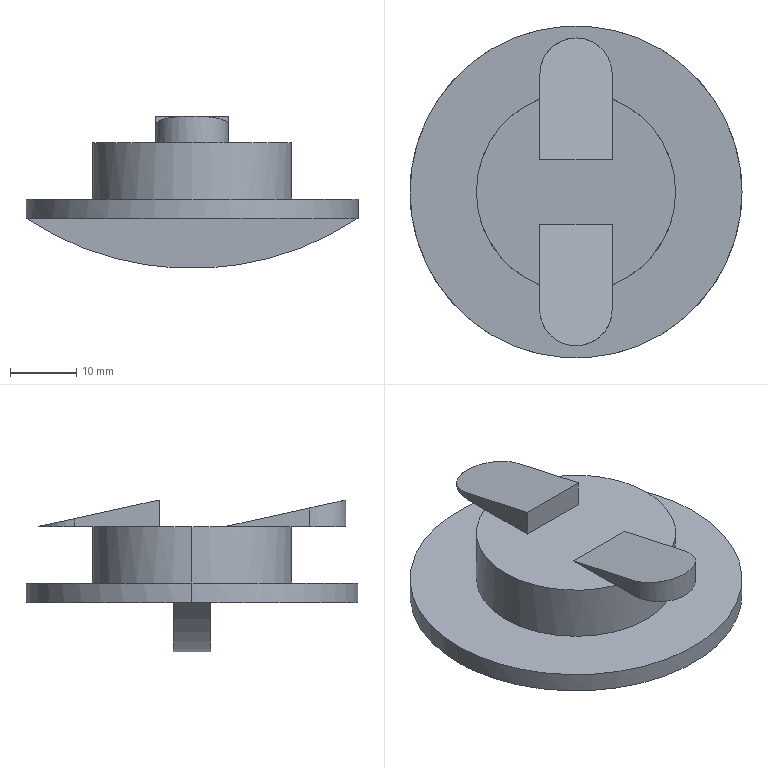Part | SolidWorks | features ICE 5, Extrusion 1 | 1 solid | 25 faces | box 50 x 50 x 22.954 mm | volume 14058 mm3 | plane 17 | cylinder 8 | commonest cylinder face diameters 10.895 x3 30 x2 50 x2 90.233 x1
STEP:
#1=CARTESIAN_POINT('',(15.,0.,10.));
#2=VERTEX_POINT('',#1);
#3=CARTESIAN_POINT('',(5.448,13.976,10.));
#4=VERTEX_POINT('',#3);
#5=CARTESIAN_POINT('',(0.,0.,10.));
#6=DIRECTION('',(0.,0.,1.));
#7=DIRECTION('',(1.,0.,0.));
#8=AXIS2_PLACEMENT_3D('',#5,#6,#7);
#9=CIRCLE('',#8,15.);
#10=EDGE_CURVE('',#2,#4,#9,.T.);
#11=ORIENTED_EDGE('',*,*,#10,.F.);
#12=CARTESIAN_POINT('',(15.,0.,1.5));
#13=VERTEX_POINT('',#12);
#14=CARTESIAN_POINT('',(15.,0.,10.));
#15=DIRECTION('',(0.,0.,-1.));
#16=VECTOR('',#15,1000.);
#17=LINE('',#14,#16);
#18=EDGE_CURVE('',#2,#13,#17,.T.);
#19=ORIENTED_EDGE('',*,*,#18,.T.);
#20=CARTESIAN_POINT('',(-15.,0.,1.5));
#21=VERTEX_POINT('',#20);
#22=CARTESIAN_POINT('',(0.,0.,1.5));
#23=DIRECTION('',(0.,0.,1.));
#24=DIRECTION('',(1.,0.,0.));
#25=AXIS2_PLACEMENT_3D('',#22,#23,#24);
#26=CIRCLE('',#25,15.);
#27=EDGE_CURVE('',#13,#21,#26,.T.);
#28=ORIENTED_EDGE('',*,*,#27,.T.);
#29=CARTESIAN_POINT('',(-15.,0.,10.));
#30=VERTEX_POINT('',#29);
#31=CARTESIAN_POINT('',(-15.,0.,10.));
#32=DIRECTION('',(0.,0.,-1.));
#33=VECTOR('',#32,1000.);
#34=LINE('',#31,#33);
#35=EDGE_CURVE('',#30,#21,#34,.T.);
#36=ORIENTED_EDGE('',*,*,#35,.F.);
#37=CARTESIAN_POINT('',(-5.448,13.976,10.));
#38=VERTEX_POINT('',#37);
#39=CARTESIAN_POINT('',(0.,0.,10.));
#40=DIRECTION('',(0.,0.,1.));
#41=DIRECTION('',(1.,0.,0.));
#42=AXIS2_PLACEMENT_3D('',#39,#40,#41);
#43=CIRCLE('',#42,15.);
#44=EDGE_CURVE('',#38,#30,#43,.T.);
#45=ORIENTED_EDGE('',*,*,#44,.F.);
#46=CARTESIAN_POINT('',(0.,0.,10.));
#47=DIRECTION('',(0.,0.,1.));
#48=DIRECTION('',(1.,0.,0.));
#49=AXIS2_PLACEMENT_3D('',#46,#47,#48);
#50=CIRCLE('',#49,15.);
#51=EDGE_CURVE('',#4,#38,#50,.T.);
#52=ORIENTED_EDGE('',*,*,#51,.F.);
#53=EDGE_LOOP('',(#11,#19,#28,#36,#45,#52));
#54=FACE_OUTER_BOUND('',#53,.T.);
#55=CARTESIAN_POINT('',(0.,0.,10.));
#56=DIRECTION('',(0.,0.,-1.));
#57=DIRECTION('',(-1.,0.,0.));
#58=AXIS2_PLACEMENT_3D('',#55,#56,#57);
#59=CYLINDRICAL_SURFACE('',#58,15.);
#60=ADVANCED_FACE('',(#54),#59,.T.);
#61=CARTESIAN_POINT('',(25.,0.,1.5));
#62=VERTEX_POINT('',#61);
#63=CARTESIAN_POINT('',(-25.,0.,1.5));
#64=VERTEX_POINT('',#63);
#65=CARTESIAN_POINT('',(0.,0.,1.5));
#66=DIRECTION('',(0.,0.,1.));
#67=DIRECTION('',(1.,0.,0.));
#68=AXIS2_PLACEMENT_3D('',#65,#66,#67);
#69=CIRCLE('',#68,25.);
#70=EDGE_CURVE('',#62,#64,#69,.T.);
#71=ORIENTED_EDGE('',*,*,#70,.F.);
#72=CARTESIAN_POINT('',(25.,0.,-1.5));
#73=VERTEX_POINT('',#72);
#74=CARTESIAN_POINT('',(25.,0.,1.5));
#75=DIRECTION('',(0.,0.,-1.));
#76=VECTOR('',#75,1000.);
#77=LINE('',#74,#76);
#78=EDGE_CURVE('',#62,#73,#77,.T.);
#79=ORIENTED_EDGE('',*,*,#78,.T.);
#80=CARTESIAN_POINT('',(24.841,2.817,-1.5));
#81=VERTEX_POINT('',#80);
#82=CARTESIAN_POINT('',(0.,0.,-1.5));
#83=DIRECTION('',(0.,0.,1.));
#84=DIRECTION('',(1.,0.,0.));
#85=AXIS2_PLACEMENT_3D('',#82,#83,#84);
#86=CIRCLE('',#85,25.);
#87=EDGE_CURVE('',#73,#81,#86,.T.);
#88=ORIENTED_EDGE('',*,*,#87,.T.);
#89=CARTESIAN_POINT('',(-24.841,2.817,-1.5));
#90=VERTEX_POINT('',#89);
#91=CARTESIAN_POINT('',(0.,0.,-1.5));
#92=DIRECTION('',(0.,0.,1.));
#93=DIRECTION('',(1.,0.,0.));
#94=AXIS2_PLACEMENT_3D('',#91,#92,#93);
#95=CIRCLE('',#94,25.);
#96=EDGE_CURVE('',#81,#90,#95,.T.);
#97=ORIENTED_EDGE('',*,*,#96,.T.);
#98=CARTESIAN_POINT('',(-25.,0.,-1.5));
#99=VERTEX_POINT('',#98);
#100=CARTESIAN_POINT('',(0.,0.,-1.5));
#101=DIRECTION('',(0.,0.,1.));
#102=DIRECTION('',(1.,0.,0.));
#103=AXIS2_PLACEMENT_3D('',#100,#101,#102);
#104=CIRCLE('',#103,25.);
#105=EDGE_CURVE('',#90,#99,#104,.T.);
#106=ORIENTED_EDGE('',*,*,#105,.T.);
#107=CARTESIAN_POINT('',(-25.,0.,1.5));
#108=DIRECTION('',(0.,0.,-1.));
#109=VECTOR('',#108,1000.);
#110=LINE('',#107,#109);
#111=EDGE_CURVE('',#64,#99,#110,.T.);
#112=ORIENTED_EDGE('',*,*,#111,.F.);
#113=EDGE_LOOP('',(#71,#79,#88,#97,#106,#112));
#114=FACE_OUTER_BOUND('',#113,.T.);
#115=CARTESIAN_POINT('',(0.,0.,1.5));
#116=DIRECTION('',(0.,0.,-1.));
#117=DIRECTION('',(-1.,0.,0.));
#118=AXIS2_PLACEMENT_3D('',#115,#116,#117);
#119=CYLINDRICAL_SURFACE('',#118,25.);
#120=ADVANCED_FACE('',(#114),#119,.T.);
#121=CARTESIAN_POINT('',(5.448,17.731,10.));
#122=VERTEX_POINT('',#121);
#123=CARTESIAN_POINT('',(0.,23.178,10.));
#124=VERTEX_POINT('',#123);
#125=CARTESIAN_POINT('',(0.,17.731,10.));
#126=DIRECTION('',(0.,0.,1.));
#127=DIRECTION('',(-1.,0.,0.));
#128=AXIS2_PLACEMENT_3D('',#125,#126,#127);
#129=CIRCLE('',#128,5.448);
#130=EDGE_CURVE('',#122,#124,#129,.T.);
#131=ORIENTED_EDGE('',*,*,#130,.T.);
#132=CARTESIAN_POINT('',(5.448,17.731,11.195));
#133=VERTEX_POINT('',#132);
#134=CARTESIAN_POINT('',(0.,23.178,10.));
#135=CARTESIAN_POINT('',(3.191,23.178,10.));
#136=CARTESIAN_POINT('',(5.448,20.922,10.495));
#137=CARTESIAN_POINT('',(5.448,17.731,11.195));
#138=(BOUNDED_CURVE()B_SPLINE_CURVE(3,(#134,#135,#136,#137),.UNSPECIFIED.,.F.,.F.)B_SPLINE_CURVE_WITH_KNOTS((4,4),(0.,1.571),.UNSPECIFIED.)CURVE()GEOMETRIC_REPRESENTATION_ITEM()RATIONAL_B_SPLINE_CURVE((1.,0.8047,0.8047,1.))REPRESENTATION_ITEM(''));
#139=EDGE_CURVE('',#124,#133,#138,.T.);
#140=ORIENTED_EDGE('',*,*,#139,.T.);
#141=CARTESIAN_POINT('',(5.448,17.731,14.));
#142=DIRECTION('',(0.,0.,-1.));
#143=VECTOR('',#142,1000.);
#144=LINE('',#141,#143);
#145=EDGE_CURVE('',#133,#122,#144,.T.);
#146=ORIENTED_EDGE('',*,*,#145,.T.);
#147=EDGE_LOOP('',(#131,#140,#146));
#148=FACE_OUTER_BOUND('',#147,.T.);
#149=CARTESIAN_POINT('',(0.,17.731,14.));
#150=DIRECTION('',(0.,0.,-1.));
#151=DIRECTION('',(-1.,0.,0.));
#152=AXIS2_PLACEMENT_3D('',#149,#150,#151);
#153=CYLINDRICAL_SURFACE('',#152,5.448);
#154=ADVANCED_FACE('',(#148),#153,.T.);
#155=CARTESIAN_POINT('',(5.448,-4.944,10.));
#156=VERTEX_POINT('',#155);
#157=CARTESIAN_POINT('',(-5.448,-4.944,10.));
#158=VERTEX_POINT('',#157);
#159=CARTESIAN_POINT('',(-5.448,-4.944,10.));
#160=DIRECTION('',(-1.,0.,0.));
#161=VECTOR('',#160,1000.);
#162=LINE('',#159,#161);
#163=EDGE_CURVE('',#156,#158,#162,.T.);
#164=ORIENTED_EDGE('',*,*,#163,.F.);
#165=CARTESIAN_POINT('',(5.448,-13.976,10.));
#166=VERTEX_POINT('',#165);
#167=CARTESIAN_POINT('',(5.448,0.,10.));
#168=DIRECTION('',(0.,-1.,0.));
#169=VECTOR('',#168,1000.);
#170=LINE('',#167,#169);
#171=EDGE_CURVE('',#156,#166,#170,.T.);
#172=ORIENTED_EDGE('',*,*,#171,.T.);
#173=CARTESIAN_POINT('',(0.,0.,10.));
#174=DIRECTION('',(0.,0.,1.));
#175=DIRECTION('',(1.,0.,0.));
#176=AXIS2_PLACEMENT_3D('',#173,#174,#175);
#177=CIRCLE('',#176,15.);
#178=EDGE_CURVE('',#166,#2,#177,.T.);
#179=ORIENTED_EDGE('',*,*,#178,.T.);
#180=ORIENTED_EDGE('',*,*,#10,.T.);
#181=CARTESIAN_POINT('',(5.448,4.944,10.));
#182=VERTEX_POINT('',#181);
#183=CARTESIAN_POINT('',(5.448,17.731,10.));
#184=DIRECTION('',(0.,1.,0.));
#185=VECTOR('',#184,1000.);
#186=LINE('',#183,#185);
#187=EDGE_CURVE('',#182,#4,#186,.T.);
#188=ORIENTED_EDGE('',*,*,#187,.F.);
#189=CARTESIAN_POINT('',(-5.448,4.944,10.));
#190=VERTEX_POINT('',#189);
#191=CARTESIAN_POINT('',(-5.448,4.944,10.));
#192=DIRECTION('',(1.,0.,0.));
#193=VECTOR('',#192,1000.);
#194=LINE('',#191,#193);
#195=EDGE_CURVE('',#190,#182,#194,.T.);
#196=ORIENTED_EDGE('',*,*,#195,.F.);
#197=CARTESIAN_POINT('',(-5.448,17.731,10.));
#198=DIRECTION('',(0.,-1.,0.));
#199=VECTOR('',#198,1000.);
#200=LINE('',#197,#199);
#201=EDGE_CURVE('',#38,#190,#200,.T.);
#202=ORIENTED_EDGE('',*,*,#201,.F.);
#203=ORIENTED_EDGE('',*,*,#44,.T.);
#204=CARTESIAN_POINT('',(-5.448,-13.976,10.));
#205=VERTEX_POINT('',#204);
#206=CARTESIAN_POINT('',(0.,0.,10.));
#207=DIRECTION('',(0.,0.,1.));
#208=DIRECTION('',(1.,0.,0.));
#209=AXIS2_PLACEMENT_3D('',#206,#207,#208);
#210=CIRCLE('',#209,15.);
#211=EDGE_CURVE('',#30,#205,#210,.T.);
#212=ORIENTED_EDGE('',*,*,#211,.T.);
#213=CARTESIAN_POINT('',(-5.448,-17.731,10.));
#214=DIRECTION('',(0.,-1.,0.));
#215=VECTOR('',#214,1000.);
#216=LINE('',#213,#215);
#217=EDGE_CURVE('',#158,#205,#216,.T.);
#218=ORIENTED_EDGE('',*,*,#217,.F.);
#219=EDGE_LOOP('',(#164,#172,#179,#180,#188,#196,#202,#203,#212,#218));
#220=FACE_OUTER_BOUND('',#219,.T.);
#221=CARTESIAN_POINT('',(0.,0.,10.));
#222=DIRECTION('',(0.,0.,1.));
#223=DIRECTION('',(1.,0.,0.));
#224=AXIS2_PLACEMENT_3D('',#221,#222,#223);
#225=PLANE('',#224);
#226=ADVANCED_FACE('',(#220),#225,.T.);
#227=CARTESIAN_POINT('',(24.841,-2.817,-1.5));
#228=VERTEX_POINT('',#227);
#229=CARTESIAN_POINT('',(-24.841,-2.817,-1.5));
#230=VERTEX_POINT('',#229);
#231=CARTESIAN_POINT('',(0.,-2.817,-1.5));
#232=DIRECTION('',(-1.,0.,0.));
#233=VECTOR('',#232,1000.);
#234=LINE('',#231,#233);
#235=EDGE_CURVE('',#228,#230,#234,.T.);
#236=ORIENTED_EDGE('',*,*,#235,.T.);
#237=CARTESIAN_POINT('',(0.,-2.817,36.162));
#238=DIRECTION('',(0.,-1.,0.));
#239=DIRECTION('',(-1.,0.,0.));
#240=AXIS2_PLACEMENT_3D('',#237,#238,#239);
#241=CIRCLE('',#240,45.116);
#242=EDGE_CURVE('',#230,#228,#241,.T.);
#243=ORIENTED_EDGE('',*,*,#242,.T.);
#244=EDGE_LOOP('',(#236,#243));
#245=FACE_OUTER_BOUND('',#244,.T.);
#246=CARTESIAN_POINT('',(0.,-2.817,-9.5));
#247=DIRECTION('',(0.,1.,0.));
#248=DIRECTION('',(-1.,0.,0.));
#249=AXIS2_PLACEMENT_3D('',#246,#247,#248);
#250=PLANE('',#249);
#251=ADVANCED_FACE('',(#245),#250,.F.);
#252=CARTESIAN_POINT('',(0.,2.817,36.162));
#253=DIRECTION('',(0.,-1.,0.));
#254=DIRECTION('',(-1.,0.,0.));
#255=AXIS2_PLACEMENT_3D('',#252,#253,#254);
#256=CIRCLE('',#255,45.116);
#257=EDGE_CURVE('',#90,#81,#256,.T.);
#258=ORIENTED_EDGE('',*,*,#257,.F.);
#259=CARTESIAN_POINT('',(0.,2.817,-1.5));
#260=DIRECTION('',(-1.,0.,0.));
#261=VECTOR('',#260,1000.);
#262=LINE('',#259,#261);
#263=EDGE_CURVE('',#81,#90,#262,.T.);
#264=ORIENTED_EDGE('',*,*,#263,.F.);
#265=EDGE_LOOP('',(#258,#264));
#266=FACE_OUTER_BOUND('',#265,.T.);
#267=CARTESIAN_POINT('',(0.,2.817,-9.5));
#268=DIRECTION('',(0.,1.,0.));
#269=DIRECTION('',(-1.,0.,0.));
#270=AXIS2_PLACEMENT_3D('',#267,#268,#269);
#271=PLANE('',#270);
#272=ADVANCED_FACE('',(#266),#271,.T.);
#273=ORIENTED_EDGE('',*,*,#235,.F.);
#274=CARTESIAN_POINT('',(0.,0.,-1.5));
#275=DIRECTION('',(0.,0.,1.));
#276=DIRECTION('',(1.,0.,0.));
#277=AXIS2_PLACEMENT_3D('',#274,#275,#276);
#278=CIRCLE('',#277,25.);
#279=EDGE_CURVE('',#230,#228,#278,.T.);
#280=ORIENTED_EDGE('',*,*,#279,.F.);
#281=EDGE_LOOP('',(#273,#280));
#282=FACE_OUTER_BOUND('',#281,.T.);
#283=CARTESIAN_POINT('',(0.,0.,-1.5));
#284=DIRECTION('',(0.,0.,1.));
#285=DIRECTION('',(1.,0.,0.));
#286=AXIS2_PLACEMENT_3D('',#283,#284,#285);
#287=PLANE('',#286);
#288=ADVANCED_FACE('',(#282),#287,.F.);
#289=ORIENTED_EDGE('',*,*,#78,.F.);
#290=CARTESIAN_POINT('',(0.,0.,1.5));
#291=DIRECTION('',(0.,0.,1.));
#292=DIRECTION('',(1.,0.,0.));
#293=AXIS2_PLACEMENT_3D('',#290,#291,#292);
#294=CIRCLE('',#293,25.);
#295=EDGE_CURVE('',#64,#62,#294,.T.);
#296=ORIENTED_EDGE('',*,*,#295,.F.);
#297=ORIENTED_EDGE('',*,*,#111,.T.);
#298=CARTESIAN_POINT('',(0.,0.,-1.5));
#299=DIRECTION('',(0.,0.,1.));
#300=DIRECTION('',(1.,0.,0.));
#301=AXIS2_PLACEMENT_3D('',#298,#299,#300);
#302=CIRCLE('',#301,25.);
#303=EDGE_CURVE('',#99,#230,#302,.T.);
#304=ORIENTED_EDGE('',*,*,#303,.T.);
#305=ORIENTED_EDGE('',*,*,#279,.T.);
#306=CARTESIAN_POINT('',(0.,0.,-1.5));
#307=DIRECTION('',(0.,0.,1.));
#308=DIRECTION('',(1.,0.,0.));
#309=AXIS2_PLACEMENT_3D('',#306,#307,#308);
#310=CIRCLE('',#309,25.);
#311=EDGE_CURVE('',#228,#73,#310,.T.);
#312=ORIENTED_EDGE('',*,*,#311,.T.);
#313=EDGE_LOOP('',(#289,#296,#297,#304,#305,#312));
#314=FACE_OUTER_BOUND('',#313,.T.);
#315=CARTESIAN_POINT('',(0.,0.,1.5));
#316=DIRECTION('',(0.,0.,-1.));
#317=DIRECTION('',(-1.,0.,0.));
#318=AXIS2_PLACEMENT_3D('',#315,#316,#317);
#319=CYLINDRICAL_SURFACE('',#318,25.);
#320=ADVANCED_FACE('',(#314),#319,.T.);
#321=CARTESIAN_POINT('',(0.,0.,1.5));
#322=DIRECTION('',(0.,0.,1.));
#323=DIRECTION('',(1.,0.,0.));
#324=AXIS2_PLACEMENT_3D('',#321,#322,#323);
#325=CIRCLE('',#324,15.);
#326=EDGE_CURVE('',#21,#13,#325,.T.);
#327=ORIENTED_EDGE('',*,*,#326,.F.);
#328=ORIENTED_EDGE('',*,*,#27,.F.);
#329=EDGE_LOOP('',(#327,#328));
#330=FACE_BOUND('',#329,.T.);
#331=ORIENTED_EDGE('',*,*,#295,.T.);
#332=ORIENTED_EDGE('',*,*,#70,.T.);
#333=EDGE_LOOP('',(#331,#332));
#334=FACE_OUTER_BOUND('',#333,.T.);
#335=CARTESIAN_POINT('',(0.,0.,1.5));
#336=DIRECTION('',(0.,0.,1.));
#337=DIRECTION('',(1.,0.,0.));
#338=AXIS2_PLACEMENT_3D('',#335,#336,#337);
#339=PLANE('',#338);
#340=ADVANCED_FACE('',(#330,#334),#339,.T.);
#341=ORIENTED_EDGE('',*,*,#96,.F.);
#342=ORIENTED_EDGE('',*,*,#263,.T.);
#343=EDGE_LOOP('',(#341,#342));
#344=FACE_OUTER_BOUND('',#343,.T.);
#345=CARTESIAN_POINT('',(0.,0.,-1.5));
#346=DIRECTION('',(0.,0.,1.));
#347=DIRECTION('',(1.,0.,0.));
#348=AXIS2_PLACEMENT_3D('',#345,#346,#347);
#349=PLANE('',#348);
#350=ADVANCED_FACE('',(#344),#349,.F.);
#351=CARTESIAN_POINT('',(-24.841,-5.183,-1.5));
#352=DIRECTION('',(0.,1.,0.));
#353=VECTOR('',#352,1000.);
#354=LINE('',#351,#353);
#355=EDGE_CURVE('',#230,#90,#354,.T.);
#356=ORIENTED_EDGE('',*,*,#355,.F.);
#357=ORIENTED_EDGE('',*,*,#303,.F.);
#358=ORIENTED_EDGE('',*,*,#105,.F.);
#359=EDGE_LOOP('',(#356,#357,#358));
#360=FACE_OUTER_BOUND('',#359,.T.);
#361=CARTESIAN_POINT('',(0.,-5.183,-1.5));
#362=DIRECTION('',(0.,0.,1.));
#363=DIRECTION('',(1.,0.,0.));
#364=AXIS2_PLACEMENT_3D('',#361,#362,#363);
#365=PLANE('',#364);
#366=ADVANCED_FACE('',(#360),#365,.F.);
#367=CARTESIAN_POINT('',(24.841,-5.183,-1.5));
#368=DIRECTION('',(0.,1.,0.));
#369=VECTOR('',#368,1000.);
#370=LINE('',#367,#369);
#371=EDGE_CURVE('',#228,#81,#370,.T.);
#372=ORIENTED_EDGE('',*,*,#371,.T.);
#373=ORIENTED_EDGE('',*,*,#87,.F.);
#374=ORIENTED_EDGE('',*,*,#311,.F.);
#375=EDGE_LOOP('',(#372,#373,#374));
#376=FACE_OUTER_BOUND('',#375,.T.);
#377=CARTESIAN_POINT('',(0.,-5.183,-1.5));
#378=DIRECTION('',(0.,0.,1.));
#379=DIRECTION('',(1.,0.,0.));
#380=AXIS2_PLACEMENT_3D('',#377,#378,#379);
#381=PLANE('',#380);
#382=ADVANCED_FACE('',(#376),#381,.F.);
#383=ORIENTED_EDGE('',*,*,#355,.T.);
#384=ORIENTED_EDGE('',*,*,#257,.T.);
#385=ORIENTED_EDGE('',*,*,#371,.F.);
#386=ORIENTED_EDGE('',*,*,#242,.F.);
#387=EDGE_LOOP('',(#383,#384,#385,#386));
#388=FACE_OUTER_BOUND('',#387,.T.);
#389=CARTESIAN_POINT('',(0.,-5.183,36.162));
#390=DIRECTION('',(0.,1.,0.));
#391=DIRECTION('',(-1.,0.,0.));
#392=AXIS2_PLACEMENT_3D('',#389,#390,#391);
#393=CYLINDRICAL_SURFACE('',#392,45.116);
#394=ADVANCED_FACE('',(#388),#393,.T.);
#395=ORIENTED_EDGE('',*,*,#18,.F.);
#396=ORIENTED_EDGE('',*,*,#178,.F.);
#397=CARTESIAN_POINT('',(0.,0.,10.));
#398=DIRECTION('',(0.,0.,1.));
#399=DIRECTION('',(1.,0.,0.));
#400=AXIS2_PLACEMENT_3D('',#397,#398,#399);
#401=CIRCLE('',#400,15.);
#402=EDGE_CURVE('',#205,#166,#401,.T.);
#403=ORIENTED_EDGE('',*,*,#402,.F.);
#404=ORIENTED_EDGE('',*,*,#211,.F.);
#405=ORIENTED_EDGE('',*,*,#35,.T.);
#406=ORIENTED_EDGE('',*,*,#326,.T.);
#407=EDGE_LOOP('',(#395,#396,#403,#404,#405,#406));
#408=FACE_OUTER_BOUND('',#407,.T.);
#409=CARTESIAN_POINT('',(0.,0.,10.));
#410=DIRECTION('',(0.,0.,-1.));
#411=DIRECTION('',(-1.,0.,0.));
#412=AXIS2_PLACEMENT_3D('',#409,#410,#411);
#413=CYLINDRICAL_SURFACE('',#412,15.);
#414=ADVANCED_FACE('',(#408),#413,.T.);
#415=ORIENTED_EDGE('',*,*,#145,.F.);
#416=CARTESIAN_POINT('',(5.448,4.944,14.));
#417=VERTEX_POINT('',#416);
#418=CARTESIAN_POINT('',(5.448,17.144,11.324));
#419=DIRECTION('',(0.,-0.9768,0.2143));
#420=VECTOR('',#419,1000.);
#421=LINE('',#418,#420);
#422=EDGE_CURVE('',#133,#417,#421,.T.);
#423=ORIENTED_EDGE('',*,*,#422,.T.);
#424=CARTESIAN_POINT('',(5.448,4.944,14.));
#425=DIRECTION('',(0.,0.,-1.));
#426=VECTOR('',#425,1000.);
#427=LINE('',#424,#426);
#428=EDGE_CURVE('',#417,#182,#427,.T.);
#429=ORIENTED_EDGE('',*,*,#428,.T.);
#430=ORIENTED_EDGE('',*,*,#187,.T.);
#431=CARTESIAN_POINT('',(5.448,17.731,10.));
#432=DIRECTION('',(0.,1.,0.));
#433=VECTOR('',#432,1000.);
#434=LINE('',#431,#433);
#435=EDGE_CURVE('',#4,#122,#434,.T.);
#436=ORIENTED_EDGE('',*,*,#435,.T.);
#437=EDGE_LOOP('',(#415,#423,#429,#430,#436));
#438=FACE_OUTER_BOUND('',#437,.T.);
#439=CARTESIAN_POINT('',(5.448,17.731,14.));
#440=DIRECTION('',(-1.,0.,0.));
#441=DIRECTION('',(0.,-1.,0.));
#442=AXIS2_PLACEMENT_3D('',#439,#440,#441);
#443=PLANE('',#442);
#444=ADVANCED_FACE('',(#438),#443,.F.);
#445=CARTESIAN_POINT('',(-5.448,17.731,11.195));
#446=VERTEX_POINT('',#445);
#447=CARTESIAN_POINT('',(-5.448,17.731,10.));
#448=VERTEX_POINT('',#447);
#449=CARTESIAN_POINT('',(-5.448,17.731,14.));
#450=DIRECTION('',(0.,0.,-1.));
#451=VECTOR('',#450,1000.);
#452=LINE('',#449,#451);
#453=EDGE_CURVE('',#446,#448,#452,.T.);
#454=ORIENTED_EDGE('',*,*,#453,.F.);
#455=CARTESIAN_POINT('',(-5.448,17.731,11.195));
#456=CARTESIAN_POINT('',(-5.448,20.922,10.495));
#457=CARTESIAN_POINT('',(-3.191,23.178,10.));
#458=CARTESIAN_POINT('',(0.,23.178,10.));
#459=(BOUNDED_CURVE()B_SPLINE_CURVE(3,(#455,#456,#457,#458),.UNSPECIFIED.,.F.,.F.)B_SPLINE_CURVE_WITH_KNOTS((4,4),(4.712,6.283),.UNSPECIFIED.)CURVE()GEOMETRIC_REPRESENTATION_ITEM()RATIONAL_B_SPLINE_CURVE((1.,0.8047,0.8047,1.))REPRESENTATION_ITEM(''));
#460=EDGE_CURVE('',#446,#124,#459,.T.);
#461=ORIENTED_EDGE('',*,*,#460,.T.);
#462=CARTESIAN_POINT('',(0.,17.731,10.));
#463=DIRECTION('',(0.,0.,1.));
#464=DIRECTION('',(-1.,0.,0.));
#465=AXIS2_PLACEMENT_3D('',#462,#463,#464);
#466=CIRCLE('',#465,5.448);
#467=EDGE_CURVE('',#124,#448,#466,.T.);
#468=ORIENTED_EDGE('',*,*,#467,.T.);
#469=EDGE_LOOP('',(#454,#461,#468));
#470=FACE_OUTER_BOUND('',#469,.T.);
#471=CARTESIAN_POINT('',(0.,17.731,14.));
#472=DIRECTION('',(0.,0.,-1.));
#473=DIRECTION('',(-1.,0.,0.));
#474=AXIS2_PLACEMENT_3D('',#471,#472,#473);
#475=CYLINDRICAL_SURFACE('',#474,5.448);
#476=ADVANCED_FACE('',(#470),#475,.T.);
#477=CARTESIAN_POINT('',(-5.448,4.944,14.));
#478=VERTEX_POINT('',#477);
#479=CARTESIAN_POINT('',(-5.448,4.944,14.));
#480=DIRECTION('',(0.,0.,-1.));
#481=VECTOR('',#480,1000.);
#482=LINE('',#479,#481);
#483=EDGE_CURVE('',#478,#190,#482,.T.);
#484=ORIENTED_EDGE('',*,*,#483,.F.);
#485=CARTESIAN_POINT('',(-5.448,23.178,10.));
#486=DIRECTION('',(0.,-0.9768,0.2143));
#487=VECTOR('',#486,1000.);
#488=LINE('',#485,#487);
#489=EDGE_CURVE('',#446,#478,#488,.T.);
#490=ORIENTED_EDGE('',*,*,#489,.F.);
#491=ORIENTED_EDGE('',*,*,#453,.T.);
#492=CARTESIAN_POINT('',(-5.448,17.731,10.));
#493=DIRECTION('',(0.,-1.,0.));
#494=VECTOR('',#493,1000.);
#495=LINE('',#492,#494);
#496=EDGE_CURVE('',#448,#38,#495,.T.);
#497=ORIENTED_EDGE('',*,*,#496,.T.);
#498=ORIENTED_EDGE('',*,*,#201,.T.);
#499=EDGE_LOOP('',(#484,#490,#491,#497,#498));
#500=FACE_OUTER_BOUND('',#499,.T.);
#501=CARTESIAN_POINT('',(-5.448,17.731,14.));
#502=DIRECTION('',(1.,0.,0.));
#503=DIRECTION('',(0.,1.,0.));
#504=AXIS2_PLACEMENT_3D('',#501,#502,#503);
#505=PLANE('',#504);
#506=ADVANCED_FACE('',(#500),#505,.F.);
#507=ORIENTED_EDGE('',*,*,#195,.T.);
#508=ORIENTED_EDGE('',*,*,#428,.F.);
#509=CARTESIAN_POINT('',(-5.448,4.944,14.));
#510=DIRECTION('',(1.,0.,0.));
#511=VECTOR('',#510,1000.);
#512=LINE('',#509,#511);
#513=EDGE_CURVE('',#478,#417,#512,.T.);
#514=ORIENTED_EDGE('',*,*,#513,.F.);
#515=ORIENTED_EDGE('',*,*,#483,.T.);
#516=EDGE_LOOP('',(#507,#508,#514,#515));
#517=FACE_OUTER_BOUND('',#516,.T.);
#518=CARTESIAN_POINT('',(-5.448,4.944,14.));
#519=DIRECTION('',(0.,1.,0.));
#520=DIRECTION('',(0.,0.,1.));
#521=AXIS2_PLACEMENT_3D('',#518,#519,#520);
#522=PLANE('',#521);
#523=ADVANCED_FACE('',(#517),#522,.F.);
#524=ORIENTED_EDGE('',*,*,#435,.F.);
#525=ORIENTED_EDGE('',*,*,#51,.T.);
#526=ORIENTED_EDGE('',*,*,#496,.F.);
#527=ORIENTED_EDGE('',*,*,#467,.F.);
#528=ORIENTED_EDGE('',*,*,#130,.F.);
#529=EDGE_LOOP('',(#524,#525,#526,#527,#528));
#530=FACE_OUTER_BOUND('',#529,.T.);
#531=CARTESIAN_POINT('',(0.,17.731,10.));
#532=DIRECTION('',(0.,0.,-1.));
#533=DIRECTION('',(-1.,0.,0.));
#534=AXIS2_PLACEMENT_3D('',#531,#532,#533);
#535=PLANE('',#534);
#536=ADVANCED_FACE('',(#530),#535,.T.);
#537=CARTESIAN_POINT('',(5.448,-17.731,12.805));
#538=VERTEX_POINT('',#537);
#539=CARTESIAN_POINT('',(5.448,-17.731,10.));
#540=VERTEX_POINT('',#539);
#541=CARTESIAN_POINT('',(5.448,-17.731,14.));
#542=DIRECTION('',(0.,0.,-1.));
#543=VECTOR('',#542,1000.);
#544=LINE('',#541,#543);
#545=EDGE_CURVE('',#538,#540,#544,.T.);
#546=ORIENTED_EDGE('',*,*,#545,.F.);
#547=CARTESIAN_POINT('',(-5.448,-17.731,12.805));
#548=VERTEX_POINT('',#547);
#549=CARTESIAN_POINT('',(5.448,-17.731,12.805));
#550=CARTESIAN_POINT('',(5.448,-28.626,15.195));
#551=CARTESIAN_POINT('',(-5.448,-28.626,15.195));
#552=CARTESIAN_POINT('',(-5.448,-17.731,12.805));
#553=(BOUNDED_CURVE()B_SPLINE_CURVE(3,(#549,#550,#551,#552),.UNSPECIFIED.,.F.,.F.)B_SPLINE_CURVE_WITH_KNOTS((4,4),(1.571,4.712),.UNSPECIFIED.)CURVE()GEOMETRIC_REPRESENTATION_ITEM()RATIONAL_B_SPLINE_CURVE((1.,0.3333,0.3333,1.))REPRESENTATION_ITEM(''));
#554=EDGE_CURVE('',#538,#548,#553,.T.);
#555=ORIENTED_EDGE('',*,*,#554,.T.);
#556=CARTESIAN_POINT('',(-5.448,-17.731,10.));
#557=VERTEX_POINT('',#556);
#558=CARTESIAN_POINT('',(-5.448,-17.731,14.));
#559=DIRECTION('',(0.,0.,-1.));
#560=VECTOR('',#559,1000.);
#561=LINE('',#558,#560);
#562=EDGE_CURVE('',#548,#557,#561,.T.);
#563=ORIENTED_EDGE('',*,*,#562,.T.);
#564=CARTESIAN_POINT('',(0.,-17.731,10.));
#565=DIRECTION('',(0.,0.,1.));
#566=DIRECTION('',(1.,0.,0.));
#567=AXIS2_PLACEMENT_3D('',#564,#565,#566);
#568=CIRCLE('',#567,5.448);
#569=EDGE_CURVE('',#557,#540,#568,.T.);
#570=ORIENTED_EDGE('',*,*,#569,.T.);
#571=EDGE_LOOP('',(#546,#555,#563,#570));
#572=FACE_OUTER_BOUND('',#571,.T.);
#573=CARTESIAN_POINT('',(0.,-17.731,14.));
#574=DIRECTION('',(0.,0.,-1.));
#575=DIRECTION('',(-1.,0.,0.));
#576=AXIS2_PLACEMENT_3D('',#573,#574,#575);
#577=CYLINDRICAL_SURFACE('',#576,5.448);
#578=ADVANCED_FACE('',(#572),#577,.T.);
#579=ORIENTED_EDGE('',*,*,#171,.F.);
#580=CARTESIAN_POINT('',(5.448,-17.981,12.86));
#581=DIRECTION('',(0.,-0.9768,0.2143));
#582=VECTOR('',#581,1000.);
#583=LINE('',#580,#582);
#584=EDGE_CURVE('',#156,#538,#583,.T.);
#585=ORIENTED_EDGE('',*,*,#584,.T.);
#586=ORIENTED_EDGE('',*,*,#545,.T.);
#587=CARTESIAN_POINT('',(5.448,-17.731,10.));
#588=DIRECTION('',(0.,1.,0.));
#589=VECTOR('',#588,1000.);
#590=LINE('',#587,#589);
#591=EDGE_CURVE('',#540,#166,#590,.T.);
#592=ORIENTED_EDGE('',*,*,#591,.T.);
#593=EDGE_LOOP('',(#579,#585,#586,#592));
#594=FACE_OUTER_BOUND('',#593,.T.);
#595=CARTESIAN_POINT('',(5.448,-17.731,14.));
#596=DIRECTION('',(-1.,0.,0.));
#597=DIRECTION('',(0.,-1.,0.));
#598=AXIS2_PLACEMENT_3D('',#595,#596,#597);
#599=PLANE('',#598);
#600=ADVANCED_FACE('',(#594),#599,.F.);
#601=ORIENTED_EDGE('',*,*,#562,.F.);
#602=CARTESIAN_POINT('',(-5.448,-23.178,14.));
#603=DIRECTION('',(0.,-0.9768,0.2143));
#604=VECTOR('',#603,1000.);
#605=LINE('',#602,#604);
#606=EDGE_CURVE('',#158,#548,#605,.T.);
#607=ORIENTED_EDGE('',*,*,#606,.F.);
#608=ORIENTED_EDGE('',*,*,#217,.T.);
#609=CARTESIAN_POINT('',(-5.448,-17.731,10.));
#610=DIRECTION('',(0.,-1.,0.));
#611=VECTOR('',#610,1000.);
#612=LINE('',#609,#611);
#613=EDGE_CURVE('',#205,#557,#612,.T.);
#614=ORIENTED_EDGE('',*,*,#613,.T.);
#615=EDGE_LOOP('',(#601,#607,#608,#614));
#616=FACE_OUTER_BOUND('',#615,.T.);
#617=CARTESIAN_POINT('',(-5.448,-17.731,14.));
#618=DIRECTION('',(1.,0.,0.));
#619=DIRECTION('',(0.,1.,0.));
#620=AXIS2_PLACEMENT_3D('',#617,#618,#619);
#621=PLANE('',#620);
#622=ADVANCED_FACE('',(#616),#621,.F.);
#623=ORIENTED_EDGE('',*,*,#613,.F.);
#624=ORIENTED_EDGE('',*,*,#402,.T.);
#625=ORIENTED_EDGE('',*,*,#591,.F.);
#626=ORIENTED_EDGE('',*,*,#569,.F.);
#627=EDGE_LOOP('',(#623,#624,#625,#626));
#628=FACE_OUTER_BOUND('',#627,.T.);
#629=CARTESIAN_POINT('',(0.,-17.731,10.));
#630=DIRECTION('',(0.,0.,1.));
#631=DIRECTION('',(1.,0.,0.));
#632=AXIS2_PLACEMENT_3D('',#629,#630,#631);
#633=PLANE('',#632);
#634=ADVANCED_FACE('',(#628),#633,.F.);
#635=ORIENTED_EDGE('',*,*,#554,.F.);
#636=ORIENTED_EDGE('',*,*,#584,.F.);
#637=ORIENTED_EDGE('',*,*,#163,.T.);
#638=ORIENTED_EDGE('',*,*,#606,.T.);
#639=EDGE_LOOP('',(#635,#636,#637,#638));
#640=FACE_OUTER_BOUND('',#639,.T.);
#641=CARTESIAN_POINT('',(25.,-23.178,14.));
#642=DIRECTION('',(0.,-0.2143,-0.9768));
#643=DIRECTION('',(0.,0.9768,-0.2143));
#644=AXIS2_PLACEMENT_3D('',#641,#642,#643);
#645=PLANE('',#644);
#646=ADVANCED_FACE('',(#640),#645,.F.);
#647=ORIENTED_EDGE('',*,*,#139,.F.);
#648=ORIENTED_EDGE('',*,*,#460,.F.);
#649=ORIENTED_EDGE('',*,*,#489,.T.);
#650=ORIENTED_EDGE('',*,*,#513,.T.);
#651=ORIENTED_EDGE('',*,*,#422,.F.);
#652=EDGE_LOOP('',(#647,#648,#649,#650,#651));
#653=FACE_OUTER_BOUND('',#652,.T.);
#654=CARTESIAN_POINT('',(25.,23.178,10.));
#655=DIRECTION('',(0.,-0.2143,-0.9768));
#656=DIRECTION('',(0.,0.9768,-0.2143));
#657=AXIS2_PLACEMENT_3D('',#654,#655,#656);
#658=PLANE('',#657);
#659=ADVANCED_FACE('',(#653),#658,.F.);
#660=CLOSED_SHELL('',(#60,#120,#154,#226,#251,#272,#288,#320,#340,#350,#366,#382,#394,#414,#444,#476,#506,#523,#536,#578,#600,#622,#634,#646,#659));
#661=MANIFOLD_SOLID_BREP('',#660);
#662=CARTESIAN_POINT('',(0.,0.,0.));
#663=DIRECTION('',(0.,0.,1.));
#664=DIRECTION('',(1.,0.,0.));
#665=AXIS2_PLACEMENT_3D('',#662,#663,#664);
#666=(LENGTH_UNIT()NAMED_UNIT(*)SI_UNIT(.MILLI.,.METRE.));
#667=UNCERTAINTY_MEASURE_WITH_UNIT(LENGTH_MEASURE(0.00001),#666,'','');
#668=(NAMED_UNIT(*)PLANE_ANGLE_UNIT()SI_UNIT($,.RADIAN.));
#669=(NAMED_UNIT(*)SI_UNIT($,.STERADIAN.)SOLID_ANGLE_UNIT());
#670=(GEOMETRIC_REPRESENTATION_CONTEXT(3)GLOBAL_UNCERTAINTY_ASSIGNED_CONTEXT((#667))GLOBAL_UNIT_ASSIGNED_CONTEXT((#666,#668,#669))REPRESENTATION_CONTEXT('',''));
#671=ADVANCED_BREP_SHAPE_REPRESENTATION('',(#661,#665),#670);